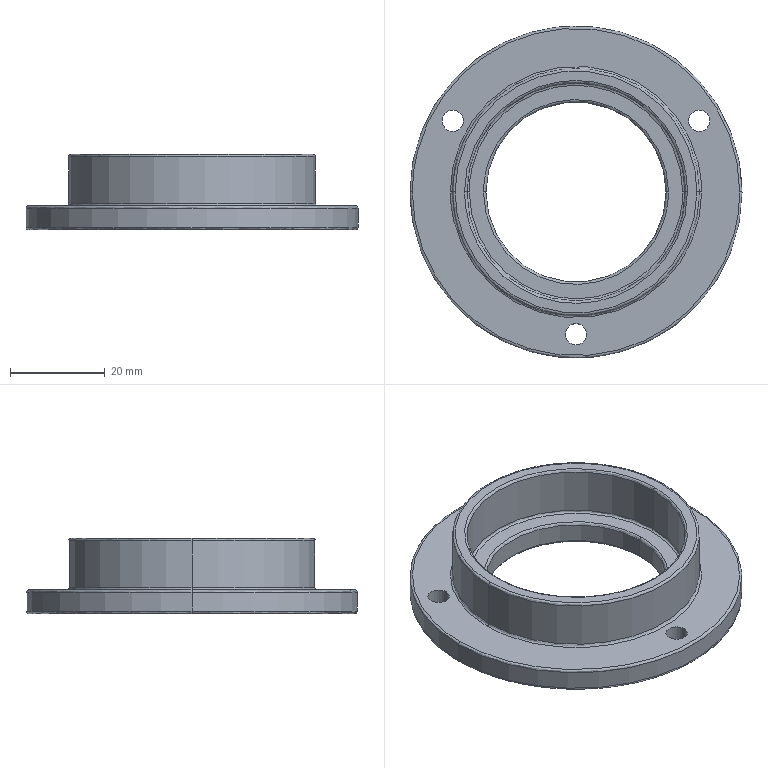Part | STEP file | Small circlip installation check head-PN_0001 | 1 solid | 34 faces | box 70 x 70 x 15.85 mm | volume 18313 mm3 | spline 16 | cylinder 14 | plane 4 | commonest cylinder face diameters 4.5 x6 38 x2 46 x2 52 x2 70 x2